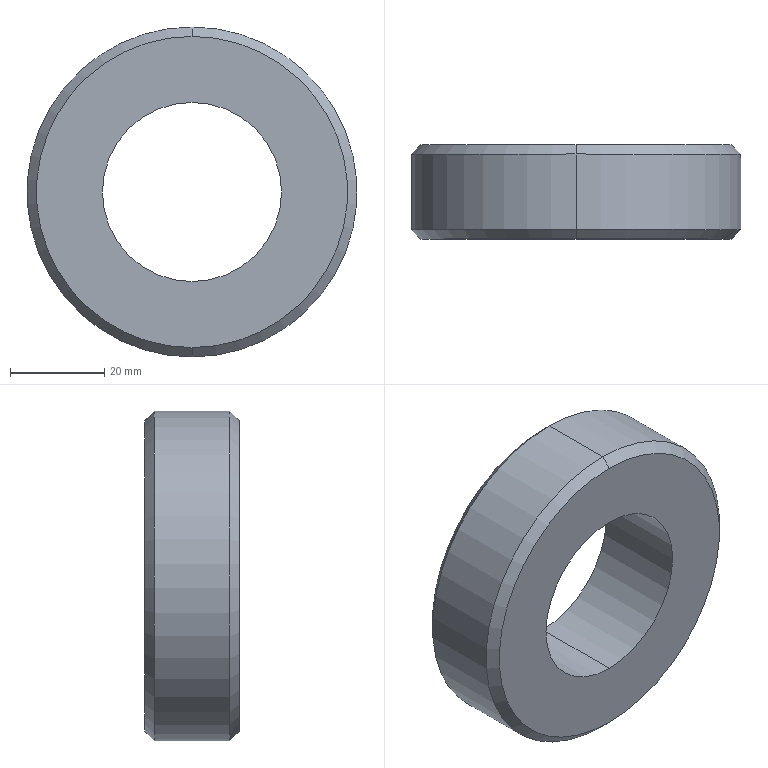Part | SolidWorks | features BaseBody 1 | 1 solid | 10 faces | box 70 x 20 x 70 mm | volume 53424 mm3 | cylinder 4 | cone 4 | plane 2 | commonest cylinder face diameters 38 x2 70 x2
STEP:
#1=CARTESIAN_POINT('',(0.,0.,-19.));
#2=VERTEX_POINT('',#1);
#3=CARTESIAN_POINT('',(0.,0.,19.));
#4=VERTEX_POINT('',#3);
#5=CARTESIAN_POINT('',(0.,0.,0.));
#6=DIRECTION('',(0.,1.,0.));
#7=DIRECTION('',(0.,0.,1.));
#8=AXIS2_PLACEMENT_3D('',#5,#6,#7);
#9=CIRCLE('',#8,19.);
#10=EDGE_CURVE('',#2,#4,#9,.T.);
#11=ORIENTED_EDGE('',*,*,#10,.F.);
#12=CARTESIAN_POINT('',(0.,20.,-19.));
#13=VERTEX_POINT('',#12);
#14=CARTESIAN_POINT('',(0.,20.,-19.));
#15=DIRECTION('',(0.,1.,0.));
#16=VECTOR('',#15,1000.);
#17=LINE('',#14,#16);
#18=EDGE_CURVE('',#2,#13,#17,.T.);
#19=ORIENTED_EDGE('',*,*,#18,.T.);
#20=CARTESIAN_POINT('',(0.,20.,19.));
#21=VERTEX_POINT('',#20);
#22=CARTESIAN_POINT('',(0.,20.,0.));
#23=DIRECTION('',(0.,1.,0.));
#24=DIRECTION('',(0.,0.,1.));
#25=AXIS2_PLACEMENT_3D('',#22,#23,#24);
#26=CIRCLE('',#25,19.);
#27=EDGE_CURVE('',#13,#21,#26,.T.);
#28=ORIENTED_EDGE('',*,*,#27,.T.);
#29=CARTESIAN_POINT('',(0.,20.,19.));
#30=DIRECTION('',(0.,1.,0.));
#31=VECTOR('',#30,1000.);
#32=LINE('',#29,#31);
#33=EDGE_CURVE('',#4,#21,#32,.T.);
#34=ORIENTED_EDGE('',*,*,#33,.F.);
#35=EDGE_LOOP('',(#11,#19,#28,#34));
#36=FACE_OUTER_BOUND('',#35,.T.);
#37=CARTESIAN_POINT('',(0.,20.,0.));
#38=DIRECTION('',(0.,1.,0.));
#39=DIRECTION('',(0.,0.,1.));
#40=AXIS2_PLACEMENT_3D('',#37,#38,#39);
#41=CYLINDRICAL_SURFACE('',#40,19.);
#42=ADVANCED_FACE('',(#36),#41,.F.);
#43=CARTESIAN_POINT('',(0.,20.,33.));
#44=VERTEX_POINT('',#43);
#45=CARTESIAN_POINT('',(0.,20.,-33.));
#46=VERTEX_POINT('',#45);
#47=CARTESIAN_POINT('',(0.,20.,0.));
#48=DIRECTION('',(0.,1.,0.));
#49=DIRECTION('',(0.,0.,1.));
#50=AXIS2_PLACEMENT_3D('',#47,#48,#49);
#51=CIRCLE('',#50,33.);
#52=EDGE_CURVE('',#44,#46,#51,.T.);
#53=ORIENTED_EDGE('',*,*,#52,.F.);
#54=CARTESIAN_POINT('',(0.,18.,35.));
#55=VERTEX_POINT('',#54);
#56=CARTESIAN_POINT('',(0.,20.,33.));
#57=DIRECTION('',(0.,-0.7071,0.7071));
#58=VECTOR('',#57,1000.);
#59=LINE('',#56,#58);
#60=EDGE_CURVE('',#44,#55,#59,.T.);
#61=ORIENTED_EDGE('',*,*,#60,.T.);
#62=CARTESIAN_POINT('',(0.,18.,-35.));
#63=VERTEX_POINT('',#62);
#64=CARTESIAN_POINT('',(0.,18.,0.));
#65=DIRECTION('',(0.,-1.,0.));
#66=DIRECTION('',(0.,0.,1.));
#67=AXIS2_PLACEMENT_3D('',#64,#65,#66);
#68=CIRCLE('',#67,35.);
#69=EDGE_CURVE('',#63,#55,#68,.T.);
#70=ORIENTED_EDGE('',*,*,#69,.F.);
#71=CARTESIAN_POINT('',(0.,20.,-33.));
#72=DIRECTION('',(0.,-0.7071,-0.7071));
#73=VECTOR('',#72,1000.);
#74=LINE('',#71,#73);
#75=EDGE_CURVE('',#46,#63,#74,.T.);
#76=ORIENTED_EDGE('',*,*,#75,.F.);
#77=EDGE_LOOP('',(#53,#61,#70,#76));
#78=FACE_OUTER_BOUND('',#77,.T.);
#79=CARTESIAN_POINT('',(0.,20.,0.));
#80=DIRECTION('',(0.,-1.,0.));
#81=DIRECTION('',(0.,0.,-1.));
#82=AXIS2_PLACEMENT_3D('',#79,#80,#81);
#83=CONICAL_SURFACE('',#82,33.,0.7854);
#84=ADVANCED_FACE('',(#78),#83,.T.);
#85=CARTESIAN_POINT('',(0.,0.,-33.));
#86=VERTEX_POINT('',#85);
#87=CARTESIAN_POINT('',(0.,0.,33.));
#88=VERTEX_POINT('',#87);
#89=CARTESIAN_POINT('',(0.,0.,0.));
#90=DIRECTION('',(0.,-1.,0.));
#91=DIRECTION('',(0.,0.,1.));
#92=AXIS2_PLACEMENT_3D('',#89,#90,#91);
#93=CIRCLE('',#92,33.);
#94=EDGE_CURVE('',#86,#88,#93,.T.);
#95=ORIENTED_EDGE('',*,*,#94,.F.);
#96=CARTESIAN_POINT('',(0.,2.,-35.));
#97=VERTEX_POINT('',#96);
#98=CARTESIAN_POINT('',(0.,2.,-35.));
#99=DIRECTION('',(0.,0.7071,-0.7071));
#100=VECTOR('',#99,1000.);
#101=LINE('',#98,#100);
#102=EDGE_CURVE('',#86,#97,#101,.T.);
#103=ORIENTED_EDGE('',*,*,#102,.T.);
#104=CARTESIAN_POINT('',(0.,2.,35.));
#105=VERTEX_POINT('',#104);
#106=CARTESIAN_POINT('',(0.,2.,0.));
#107=DIRECTION('',(0.,1.,0.));
#108=DIRECTION('',(0.,0.,1.));
#109=AXIS2_PLACEMENT_3D('',#106,#107,#108);
#110=CIRCLE('',#109,35.);
#111=EDGE_CURVE('',#105,#97,#110,.T.);
#112=ORIENTED_EDGE('',*,*,#111,.F.);
#113=CARTESIAN_POINT('',(0.,2.,35.));
#114=DIRECTION('',(0.,0.7071,0.7071));
#115=VECTOR('',#114,1000.);
#116=LINE('',#113,#115);
#117=EDGE_CURVE('',#88,#105,#116,.T.);
#118=ORIENTED_EDGE('',*,*,#117,.F.);
#119=EDGE_LOOP('',(#95,#103,#112,#118));
#120=FACE_OUTER_BOUND('',#119,.T.);
#121=CARTESIAN_POINT('',(0.,2.,0.));
#122=DIRECTION('',(0.,1.,0.));
#123=DIRECTION('',(0.,0.,1.));
#124=AXIS2_PLACEMENT_3D('',#121,#122,#123);
#125=CONICAL_SURFACE('',#124,35.,0.7854);
#126=ADVANCED_FACE('',(#120),#125,.T.);
#127=ORIENTED_EDGE('',*,*,#69,.T.);
#128=CARTESIAN_POINT('',(0.,20.,35.));
#129=DIRECTION('',(0.,-1.,0.));
#130=VECTOR('',#129,1000.);
#131=LINE('',#128,#130);
#132=EDGE_CURVE('',#55,#105,#131,.T.);
#133=ORIENTED_EDGE('',*,*,#132,.T.);
#134=ORIENTED_EDGE('',*,*,#111,.T.);
#135=CARTESIAN_POINT('',(0.,20.,-35.));
#136=DIRECTION('',(0.,-1.,0.));
#137=VECTOR('',#136,1000.);
#138=LINE('',#135,#137);
#139=EDGE_CURVE('',#63,#97,#138,.T.);
#140=ORIENTED_EDGE('',*,*,#139,.F.);
#141=EDGE_LOOP('',(#127,#133,#134,#140));
#142=FACE_OUTER_BOUND('',#141,.T.);
#143=CARTESIAN_POINT('',(0.,20.,0.));
#144=DIRECTION('',(0.,-1.,0.));
#145=DIRECTION('',(0.,0.,-1.));
#146=AXIS2_PLACEMENT_3D('',#143,#144,#145);
#147=CYLINDRICAL_SURFACE('',#146,35.);
#148=ADVANCED_FACE('',(#142),#147,.T.);
#149=ORIENTED_EDGE('',*,*,#132,.F.);
#150=CARTESIAN_POINT('',(0.,18.,0.));
#151=DIRECTION('',(0.,-1.,0.));
#152=DIRECTION('',(0.,0.,1.));
#153=AXIS2_PLACEMENT_3D('',#150,#151,#152);
#154=CIRCLE('',#153,35.);
#155=EDGE_CURVE('',#55,#63,#154,.T.);
#156=ORIENTED_EDGE('',*,*,#155,.T.);
#157=ORIENTED_EDGE('',*,*,#139,.T.);
#158=CARTESIAN_POINT('',(0.,2.,0.));
#159=DIRECTION('',(0.,1.,0.));
#160=DIRECTION('',(0.,0.,1.));
#161=AXIS2_PLACEMENT_3D('',#158,#159,#160);
#162=CIRCLE('',#161,35.);
#163=EDGE_CURVE('',#97,#105,#162,.T.);
#164=ORIENTED_EDGE('',*,*,#163,.T.);
#165=EDGE_LOOP('',(#149,#156,#157,#164));
#166=FACE_OUTER_BOUND('',#165,.T.);
#167=CARTESIAN_POINT('',(0.,20.,0.));
#168=DIRECTION('',(0.,-1.,0.));
#169=DIRECTION('',(0.,0.,-1.));
#170=AXIS2_PLACEMENT_3D('',#167,#168,#169);
#171=CYLINDRICAL_SURFACE('',#170,35.);
#172=ADVANCED_FACE('',(#166),#171,.T.);
#173=CARTESIAN_POINT('',(0.,20.,0.));
#174=DIRECTION('',(0.,1.,0.));
#175=DIRECTION('',(0.,0.,1.));
#176=AXIS2_PLACEMENT_3D('',#173,#174,#175);
#177=CIRCLE('',#176,19.);
#178=EDGE_CURVE('',#21,#13,#177,.T.);
#179=ORIENTED_EDGE('',*,*,#178,.F.);
#180=ORIENTED_EDGE('',*,*,#27,.F.);
#181=EDGE_LOOP('',(#179,#180));
#182=FACE_BOUND('',#181,.T.);
#183=CARTESIAN_POINT('',(0.,20.,0.));
#184=DIRECTION('',(0.,1.,0.));
#185=DIRECTION('',(0.,0.,1.));
#186=AXIS2_PLACEMENT_3D('',#183,#184,#185);
#187=CIRCLE('',#186,33.);
#188=EDGE_CURVE('',#46,#44,#187,.T.);
#189=ORIENTED_EDGE('',*,*,#188,.T.);
#190=ORIENTED_EDGE('',*,*,#52,.T.);
#191=EDGE_LOOP('',(#189,#190));
#192=FACE_OUTER_BOUND('',#191,.T.);
#193=CARTESIAN_POINT('',(0.,20.,0.));
#194=DIRECTION('',(0.,1.,0.));
#195=DIRECTION('',(0.,0.,1.));
#196=AXIS2_PLACEMENT_3D('',#193,#194,#195);
#197=PLANE('',#196);
#198=ADVANCED_FACE('',(#182,#192),#197,.T.);
#199=CARTESIAN_POINT('',(0.,0.,0.));
#200=DIRECTION('',(0.,1.,0.));
#201=DIRECTION('',(0.,0.,1.));
#202=AXIS2_PLACEMENT_3D('',#199,#200,#201);
#203=CIRCLE('',#202,19.);
#204=EDGE_CURVE('',#4,#2,#203,.T.);
#205=ORIENTED_EDGE('',*,*,#204,.T.);
#206=ORIENTED_EDGE('',*,*,#10,.T.);
#207=EDGE_LOOP('',(#205,#206));
#208=FACE_BOUND('',#207,.T.);
#209=CARTESIAN_POINT('',(0.,0.,0.));
#210=DIRECTION('',(0.,-1.,0.));
#211=DIRECTION('',(0.,0.,1.));
#212=AXIS2_PLACEMENT_3D('',#209,#210,#211);
#213=CIRCLE('',#212,33.);
#214=EDGE_CURVE('',#88,#86,#213,.T.);
#215=ORIENTED_EDGE('',*,*,#214,.T.);
#216=ORIENTED_EDGE('',*,*,#94,.T.);
#217=EDGE_LOOP('',(#215,#216));
#218=FACE_OUTER_BOUND('',#217,.T.);
#219=CARTESIAN_POINT('',(0.,0.,0.));
#220=DIRECTION('',(0.,1.,0.));
#221=DIRECTION('',(0.,0.,1.));
#222=AXIS2_PLACEMENT_3D('',#219,#220,#221);
#223=PLANE('',#222);
#224=ADVANCED_FACE('',(#208,#218),#223,.F.);
#225=ORIENTED_EDGE('',*,*,#102,.F.);
#226=ORIENTED_EDGE('',*,*,#214,.F.);
#227=ORIENTED_EDGE('',*,*,#117,.T.);
#228=ORIENTED_EDGE('',*,*,#163,.F.);
#229=EDGE_LOOP('',(#225,#226,#227,#228));
#230=FACE_OUTER_BOUND('',#229,.T.);
#231=CARTESIAN_POINT('',(0.,2.,0.));
#232=DIRECTION('',(0.,1.,0.));
#233=DIRECTION('',(0.,0.,1.));
#234=AXIS2_PLACEMENT_3D('',#231,#232,#233);
#235=CONICAL_SURFACE('',#234,35.,0.7854);
#236=ADVANCED_FACE('',(#230),#235,.T.);
#237=ORIENTED_EDGE('',*,*,#60,.F.);
#238=ORIENTED_EDGE('',*,*,#188,.F.);
#239=ORIENTED_EDGE('',*,*,#75,.T.);
#240=ORIENTED_EDGE('',*,*,#155,.F.);
#241=EDGE_LOOP('',(#237,#238,#239,#240));
#242=FACE_OUTER_BOUND('',#241,.T.);
#243=CARTESIAN_POINT('',(0.,20.,0.));
#244=DIRECTION('',(0.,-1.,0.));
#245=DIRECTION('',(0.,0.,-1.));
#246=AXIS2_PLACEMENT_3D('',#243,#244,#245);
#247=CONICAL_SURFACE('',#246,33.,0.7854);
#248=ADVANCED_FACE('',(#242),#247,.T.);
#249=ORIENTED_EDGE('',*,*,#18,.F.);
#250=ORIENTED_EDGE('',*,*,#204,.F.);
#251=ORIENTED_EDGE('',*,*,#33,.T.);
#252=ORIENTED_EDGE('',*,*,#178,.T.);
#253=EDGE_LOOP('',(#249,#250,#251,#252));
#254=FACE_OUTER_BOUND('',#253,.T.);
#255=CARTESIAN_POINT('',(0.,20.,0.));
#256=DIRECTION('',(0.,1.,0.));
#257=DIRECTION('',(0.,0.,1.));
#258=AXIS2_PLACEMENT_3D('',#255,#256,#257);
#259=CYLINDRICAL_SURFACE('',#258,19.);
#260=ADVANCED_FACE('',(#254),#259,.F.);
#261=CLOSED_SHELL('',(#42,#84,#126,#148,#172,#198,#224,#236,#248,#260));
#262=MANIFOLD_SOLID_BREP('',#261);
#263=CARTESIAN_POINT('',(0.,0.,0.));
#264=DIRECTION('',(0.,0.,1.));
#265=DIRECTION('',(1.,0.,0.));
#266=AXIS2_PLACEMENT_3D('',#263,#264,#265);
#267=(LENGTH_UNIT()NAMED_UNIT(*)SI_UNIT(.MILLI.,.METRE.));
#268=UNCERTAINTY_MEASURE_WITH_UNIT(LENGTH_MEASURE(0.00001),#267,'','');
#269=(NAMED_UNIT(*)PLANE_ANGLE_UNIT()SI_UNIT($,.RADIAN.));
#270=(NAMED_UNIT(*)SI_UNIT($,.STERADIAN.)SOLID_ANGLE_UNIT());
#271=(GEOMETRIC_REPRESENTATION_CONTEXT(3)GLOBAL_UNCERTAINTY_ASSIGNED_CONTEXT((#268))GLOBAL_UNIT_ASSIGNED_CONTEXT((#267,#269,#270))REPRESENTATION_CONTEXT('',''));
#272=ADVANCED_BREP_SHAPE_REPRESENTATION('',(#262,#266),#271);